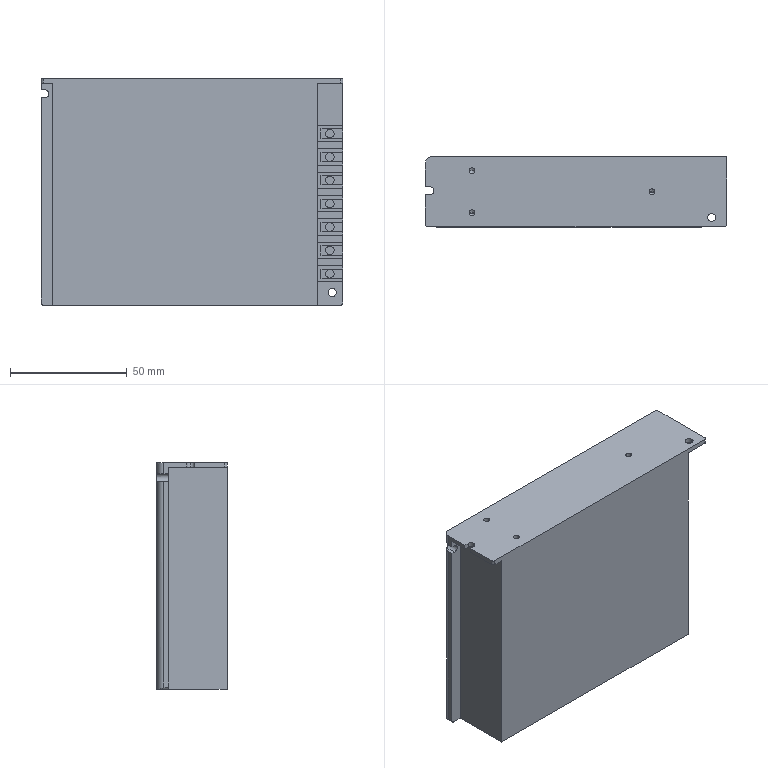Part | STEP file | Switching power supply LRS-100-48 | 1 solid | 128 faces | box 129 x 30 x 97 mm | volume 340596 mm3 | plane 81 | cylinder 37 | cone 10 | commonest cylinder face diameters 3.666 x14 2.5 x10 2 x4 3.4 x4 3.5 x3 6 x2